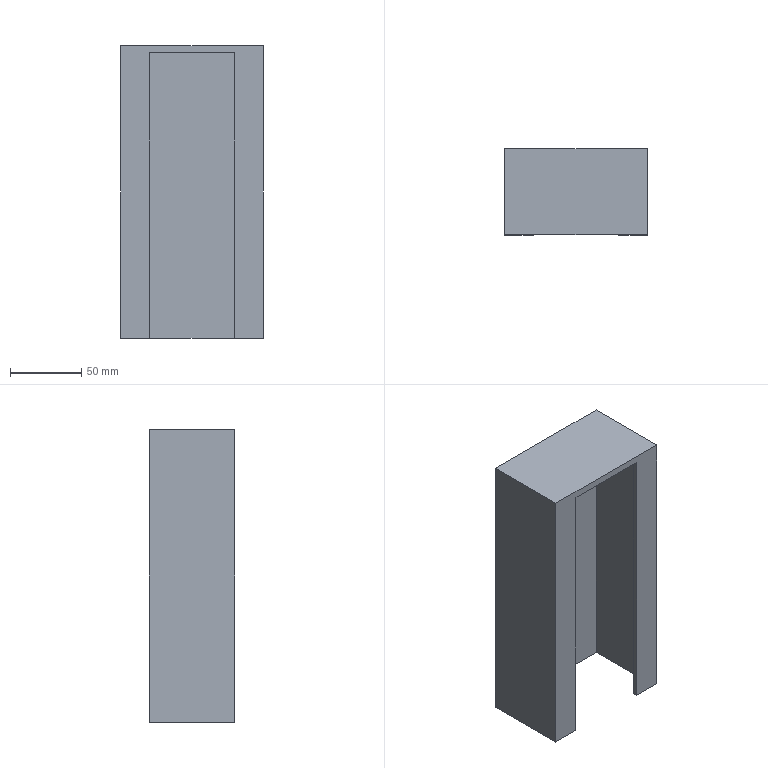Part | STEP file | 1 solid | 14 faces | box 100 x 60 x 205 mm | volume 178800 mm3 | plane 14
STEP:
#1=CARTESIAN_POINT('',(0.,0.,0.));
#2=DIRECTION('',(0.,0.,1.));
#3=DIRECTION('',(1.,0.,0.));
#4=AXIS2_PLACEMENT_3D('',#1,#2,#3);
#5=CARTESIAN_POINT('',(-50.,45.812,205.));
#6=VERTEX_POINT('',#5);
#7=CARTESIAN_POINT('',(50.,45.812,205.));
#8=VERTEX_POINT('',#7);
#9=CARTESIAN_POINT('',(50.,45.812,205.));
#10=DIRECTION('',(1.,0.,0.));
#11=VECTOR('',#10,1.);
#12=LINE('',#9,#11);
#13=CARTESIAN_POINT('',(50.,45.812,0.));
#14=DIRECTION('',(0.,1.,0.));
#15=DIRECTION('',(0.,0.,1.));
#16=AXIS2_PLACEMENT_3D('',#13,#14,#15);
#17=PLANE('',#16);
#18=CARTESIAN_POINT('',(205.,0.));
#19=DIRECTION('',(0.,1.));
#20=VECTOR('',#19,1.);
#21=LINE('',#18,#20);
#22=(GEOMETRIC_REPRESENTATION_CONTEXT(2)PARAMETRIC_REPRESENTATION_CONTEXT()REPRESENTATION_CONTEXT('',''));
#23=DEFINITIONAL_REPRESENTATION('',(#21),#22);
#24=PCURVE('',#17,#23);
#25=CARTESIAN_POINT('',(0.,15.812,205.));
#26=DIRECTION('',(0.,0.,1.));
#27=DIRECTION('',(1.,0.,0.));
#28=AXIS2_PLACEMENT_3D('',#25,#26,#27);
#29=PLANE('',#28);
#30=CARTESIAN_POINT('',(50.,30.));
#31=DIRECTION('',(1.,0.));
#32=VECTOR('',#31,1.);
#33=LINE('',#30,#32);
#34=(GEOMETRIC_REPRESENTATION_CONTEXT(2)PARAMETRIC_REPRESENTATION_CONTEXT()REPRESENTATION_CONTEXT('',''));
#35=DEFINITIONAL_REPRESENTATION('',(#33),#34);
#36=PCURVE('',#29,#35);
#37=SURFACE_CURVE('',#12,(#24,#36),.PCURVE_S1.);
#38=EDGE_CURVE('',#6,#8,#37,.T.);
#39=ORIENTED_EDGE('',*,*,#38,.T.);
#40=CARTESIAN_POINT('',(50.,45.812,0.));
#41=VERTEX_POINT('',#40);
#42=CARTESIAN_POINT('',(50.,45.812,0.));
#43=DIRECTION('',(0.,0.,-1.));
#44=VECTOR('',#43,1.);
#45=LINE('',#42,#44);
#46=CARTESIAN_POINT('',(0.,0.));
#47=DIRECTION('',(-1.,0.));
#48=VECTOR('',#47,1.);
#49=LINE('',#46,#48);
#50=(GEOMETRIC_REPRESENTATION_CONTEXT(2)PARAMETRIC_REPRESENTATION_CONTEXT()REPRESENTATION_CONTEXT('',''));
#51=DEFINITIONAL_REPRESENTATION('',(#49),#50);
#52=PCURVE('',#17,#51);
#53=CARTESIAN_POINT('',(50.,-14.188,0.));
#54=DIRECTION('',(1.,0.,0.));
#55=DIRECTION('',(0.,1.,0.));
#56=AXIS2_PLACEMENT_3D('',#53,#54,#55);
#57=PLANE('',#56);
#58=CARTESIAN_POINT('',(60.,0.));
#59=DIRECTION('',(0.,-1.));
#60=VECTOR('',#59,1.);
#61=LINE('',#58,#60);
#62=(GEOMETRIC_REPRESENTATION_CONTEXT(2)PARAMETRIC_REPRESENTATION_CONTEXT()REPRESENTATION_CONTEXT('',''));
#63=DEFINITIONAL_REPRESENTATION('',(#61),#62);
#64=PCURVE('',#57,#63);
#65=SURFACE_CURVE('',#45,(#52,#64),.PCURVE_S1.);
#66=EDGE_CURVE('',#8,#41,#65,.T.);
#67=ORIENTED_EDGE('',*,*,#66,.T.);
#68=CARTESIAN_POINT('',(-50.,45.812,0.));
#69=VERTEX_POINT('',#68);
#70=CARTESIAN_POINT('',(50.,45.812,0.));
#71=DIRECTION('',(-1.,0.,0.));
#72=VECTOR('',#71,1.);
#73=LINE('',#70,#72);
#74=CARTESIAN_POINT('',(0.,0.));
#75=DIRECTION('',(0.,-1.));
#76=VECTOR('',#75,1.);
#77=LINE('',#74,#76);
#78=(GEOMETRIC_REPRESENTATION_CONTEXT(2)PARAMETRIC_REPRESENTATION_CONTEXT()REPRESENTATION_CONTEXT('',''));
#79=DEFINITIONAL_REPRESENTATION('',(#77),#78);
#80=PCURVE('',#17,#79);
#81=CARTESIAN_POINT('',(0.,22.284,0.));
#82=DIRECTION('',(0.,0.,1.));
#83=DIRECTION('',(1.,0.,0.));
#84=AXIS2_PLACEMENT_3D('',#81,#82,#83);
#85=PLANE('',#84);
#86=CARTESIAN_POINT('',(50.,23.528));
#87=DIRECTION('',(-1.,0.));
#88=VECTOR('',#87,1.);
#89=LINE('',#86,#88);
#90=(GEOMETRIC_REPRESENTATION_CONTEXT(2)PARAMETRIC_REPRESENTATION_CONTEXT()REPRESENTATION_CONTEXT('',''));
#91=DEFINITIONAL_REPRESENTATION('',(#89),#90);
#92=PCURVE('',#85,#91);
#93=SURFACE_CURVE('',#73,(#80,#92),.PCURVE_S1.);
#94=EDGE_CURVE('',#41,#69,#93,.T.);
#95=ORIENTED_EDGE('',*,*,#94,.T.);
#96=CARTESIAN_POINT('',(-50.,45.812,0.));
#97=DIRECTION('',(0.,0.,1.));
#98=VECTOR('',#97,1.);
#99=LINE('',#96,#98);
#100=CARTESIAN_POINT('',(0.,-100.));
#101=DIRECTION('',(1.,0.));
#102=VECTOR('',#101,1.);
#103=LINE('',#100,#102);
#104=(GEOMETRIC_REPRESENTATION_CONTEXT(2)PARAMETRIC_REPRESENTATION_CONTEXT()REPRESENTATION_CONTEXT('',''));
#105=DEFINITIONAL_REPRESENTATION('',(#103),#104);
#106=PCURVE('',#17,#105);
#107=CARTESIAN_POINT('',(-50.,45.812,0.));
#108=DIRECTION('',(-1.,0.,0.));
#109=DIRECTION('',(0.,-1.,0.));
#110=AXIS2_PLACEMENT_3D('',#107,#108,#109);
#111=PLANE('',#110);
#112=CARTESIAN_POINT('',(0.,0.));
#113=DIRECTION('',(0.,1.));
#114=VECTOR('',#113,1.);
#115=LINE('',#112,#114);
#116=(GEOMETRIC_REPRESENTATION_CONTEXT(2)PARAMETRIC_REPRESENTATION_CONTEXT()REPRESENTATION_CONTEXT('',''));
#117=DEFINITIONAL_REPRESENTATION('',(#115),#116);
#118=PCURVE('',#111,#117);
#119=SURFACE_CURVE('',#99,(#106,#118),.PCURVE_S1.);
#120=EDGE_CURVE('',#69,#6,#119,.T.);
#121=ORIENTED_EDGE('',*,*,#120,.T.);
#122=EDGE_LOOP('',(#39,#67,#95,#121));
#123=FACE_BOUND('',#122,.T.);
#124=ADVANCED_FACE('',(#123),#17,.T.);
#125=CARTESIAN_POINT('',(50.,-14.188,205.));
#126=VERTEX_POINT('',#125);
#127=CARTESIAN_POINT('',(50.,-14.188,205.));
#128=DIRECTION('',(0.,-1.,0.));
#129=VECTOR('',#128,1.);
#130=LINE('',#127,#129);
#131=CARTESIAN_POINT('',(0.,205.));
#132=DIRECTION('',(-1.,0.));
#133=VECTOR('',#132,1.);
#134=LINE('',#131,#133);
#135=(GEOMETRIC_REPRESENTATION_CONTEXT(2)PARAMETRIC_REPRESENTATION_CONTEXT()REPRESENTATION_CONTEXT('',''));
#136=DEFINITIONAL_REPRESENTATION('',(#134),#135);
#137=PCURVE('',#57,#136);
#138=CARTESIAN_POINT('',(50.,-30.));
#139=DIRECTION('',(0.,-1.));
#140=VECTOR('',#139,1.);
#141=LINE('',#138,#140);
#142=(GEOMETRIC_REPRESENTATION_CONTEXT(2)PARAMETRIC_REPRESENTATION_CONTEXT()REPRESENTATION_CONTEXT('',''));
#143=DEFINITIONAL_REPRESENTATION('',(#141),#142);
#144=PCURVE('',#29,#143);
#145=SURFACE_CURVE('',#130,(#137,#144),.PCURVE_S1.);
#146=EDGE_CURVE('',#8,#126,#145,.T.);
#147=ORIENTED_EDGE('',*,*,#146,.T.);
#148=CARTESIAN_POINT('',(50.,-14.188,0.));
#149=VERTEX_POINT('',#148);
#150=CARTESIAN_POINT('',(50.,-14.188,0.));
#151=DIRECTION('',(0.,0.,-1.));
#152=VECTOR('',#151,1.);
#153=LINE('',#150,#152);
#154=CARTESIAN_POINT('',(0.,0.));
#155=DIRECTION('',(0.,-1.));
#156=VECTOR('',#155,1.);
#157=LINE('',#154,#156);
#158=(GEOMETRIC_REPRESENTATION_CONTEXT(2)PARAMETRIC_REPRESENTATION_CONTEXT()REPRESENTATION_CONTEXT('',''));
#159=DEFINITIONAL_REPRESENTATION('',(#157),#158);
#160=PCURVE('',#57,#159);
#161=CARTESIAN_POINT('',(30.,-14.188,0.));
#162=DIRECTION('',(0.,-1.,0.));
#163=DIRECTION('',(1.,0.,0.));
#164=AXIS2_PLACEMENT_3D('',#161,#162,#163);
#165=PLANE('',#164);
#166=CARTESIAN_POINT('',(20.,0.));
#167=DIRECTION('',(0.,-1.));
#168=VECTOR('',#167,1.);
#169=LINE('',#166,#168);
#170=(GEOMETRIC_REPRESENTATION_CONTEXT(2)PARAMETRIC_REPRESENTATION_CONTEXT()REPRESENTATION_CONTEXT('',''));
#171=DEFINITIONAL_REPRESENTATION('',(#169),#170);
#172=PCURVE('',#165,#171);
#173=SURFACE_CURVE('',#153,(#160,#172),.PCURVE_S1.);
#174=EDGE_CURVE('',#126,#149,#173,.T.);
#175=ORIENTED_EDGE('',*,*,#174,.T.);
#176=CARTESIAN_POINT('',(50.,-14.188,0.));
#177=DIRECTION('',(0.,1.,0.));
#178=VECTOR('',#177,1.);
#179=LINE('',#176,#178);
#180=CARTESIAN_POINT('',(0.,0.));
#181=DIRECTION('',(1.,0.));
#182=VECTOR('',#181,1.);
#183=LINE('',#180,#182);
#184=(GEOMETRIC_REPRESENTATION_CONTEXT(2)PARAMETRIC_REPRESENTATION_CONTEXT()REPRESENTATION_CONTEXT('',''));
#185=DEFINITIONAL_REPRESENTATION('',(#183),#184);
#186=PCURVE('',#57,#185);
#187=CARTESIAN_POINT('',(50.,-36.472));
#188=DIRECTION('',(0.,1.));
#189=VECTOR('',#188,1.);
#190=LINE('',#187,#189);
#191=(GEOMETRIC_REPRESENTATION_CONTEXT(2)PARAMETRIC_REPRESENTATION_CONTEXT()REPRESENTATION_CONTEXT('',''));
#192=DEFINITIONAL_REPRESENTATION('',(#190),#191);
#193=PCURVE('',#85,#192);
#194=SURFACE_CURVE('',#179,(#186,#193),.PCURVE_S1.);
#195=EDGE_CURVE('',#149,#41,#194,.T.);
#196=ORIENTED_EDGE('',*,*,#195,.T.);
#197=ORIENTED_EDGE('',*,*,#66,.F.);
#198=EDGE_LOOP('',(#147,#175,#196,#197));
#199=FACE_BOUND('',#198,.T.);
#200=ADVANCED_FACE('',(#199),#57,.T.);
#201=ORIENTED_EDGE('',*,*,#146,.F.);
#202=ORIENTED_EDGE('',*,*,#38,.F.);
#203=CARTESIAN_POINT('',(-50.,-14.188,205.));
#204=VERTEX_POINT('',#203);
#205=CARTESIAN_POINT('',(-50.,15.812,205.));
#206=DIRECTION('',(0.,-1.,0.));
#207=VECTOR('',#206,1.);
#208=LINE('',#205,#207);
#209=CARTESIAN_POINT('',(-50.,0.));
#210=DIRECTION('',(0.,-1.));
#211=VECTOR('',#210,1.);
#212=LINE('',#209,#211);
#213=(GEOMETRIC_REPRESENTATION_CONTEXT(2)PARAMETRIC_REPRESENTATION_CONTEXT()REPRESENTATION_CONTEXT('',''));
#214=DEFINITIONAL_REPRESENTATION('',(#212),#213);
#215=PCURVE('',#29,#214);
#216=CARTESIAN_POINT('',(30.,205.));
#217=DIRECTION('',(1.,0.));
#218=VECTOR('',#217,1.);
#219=LINE('',#216,#218);
#220=(GEOMETRIC_REPRESENTATION_CONTEXT(2)PARAMETRIC_REPRESENTATION_CONTEXT()REPRESENTATION_CONTEXT('',''));
#221=DEFINITIONAL_REPRESENTATION('',(#219),#220);
#222=PCURVE('',#111,#221);
#223=SURFACE_CURVE('',#208,(#215,#222),.PCURVE_S1.);
#224=EDGE_CURVE('',#6,#204,#223,.T.);
#225=ORIENTED_EDGE('',*,*,#224,.T.);
#226=CARTESIAN_POINT('',(0.,-14.188,205.));
#227=DIRECTION('',(1.,0.,0.));
#228=VECTOR('',#227,1.);
#229=LINE('',#226,#228);
#230=CARTESIAN_POINT('',(0.,-30.));
#231=DIRECTION('',(1.,0.));
#232=VECTOR('',#231,1.);
#233=LINE('',#230,#232);
#234=(GEOMETRIC_REPRESENTATION_CONTEXT(2)PARAMETRIC_REPRESENTATION_CONTEXT()REPRESENTATION_CONTEXT('',''));
#235=DEFINITIONAL_REPRESENTATION('',(#233),#234);
#236=PCURVE('',#29,#235);
#237=CARTESIAN_POINT('',(-30.,205.));
#238=DIRECTION('',(1.,0.));
#239=VECTOR('',#238,1.);
#240=LINE('',#237,#239);
#241=(GEOMETRIC_REPRESENTATION_CONTEXT(2)PARAMETRIC_REPRESENTATION_CONTEXT()REPRESENTATION_CONTEXT('',''));
#242=DEFINITIONAL_REPRESENTATION('',(#240),#241);
#243=PCURVE('',#165,#242);
#244=SURFACE_CURVE('',#229,(#236,#243),.PCURVE_S1.);
#245=EDGE_CURVE('',#204,#126,#244,.T.);
#246=ORIENTED_EDGE('',*,*,#245,.T.);
#247=EDGE_LOOP('',(#201,#202,#225,#246));
#248=FACE_BOUND('',#247,.T.);
#249=ADVANCED_FACE('',(#248),#29,.T.);
#250=ORIENTED_EDGE('',*,*,#224,.F.);
#251=ORIENTED_EDGE('',*,*,#120,.F.);
#252=CARTESIAN_POINT('',(-50.,-14.188,0.));
#253=VERTEX_POINT('',#252);
#254=CARTESIAN_POINT('',(-50.,45.812,0.));
#255=DIRECTION('',(0.,-1.,0.));
#256=VECTOR('',#255,1.);
#257=LINE('',#254,#256);
#258=CARTESIAN_POINT('',(0.,0.));
#259=DIRECTION('',(1.,0.));
#260=VECTOR('',#259,1.);
#261=LINE('',#258,#260);
#262=(GEOMETRIC_REPRESENTATION_CONTEXT(2)PARAMETRIC_REPRESENTATION_CONTEXT()REPRESENTATION_CONTEXT('',''));
#263=DEFINITIONAL_REPRESENTATION('',(#261),#262);
#264=PCURVE('',#111,#263);
#265=CARTESIAN_POINT('',(-50.,23.528));
#266=DIRECTION('',(0.,-1.));
#267=VECTOR('',#266,1.);
#268=LINE('',#265,#267);
#269=(GEOMETRIC_REPRESENTATION_CONTEXT(2)PARAMETRIC_REPRESENTATION_CONTEXT()REPRESENTATION_CONTEXT('',''));
#270=DEFINITIONAL_REPRESENTATION('',(#268),#269);
#271=PCURVE('',#85,#270);
#272=SURFACE_CURVE('',#257,(#264,#271),.PCURVE_S1.);
#273=EDGE_CURVE('',#69,#253,#272,.T.);
#274=ORIENTED_EDGE('',*,*,#273,.T.);
#275=CARTESIAN_POINT('',(-50.,-14.188,0.));
#276=DIRECTION('',(0.,0.,1.));
#277=VECTOR('',#276,1.);
#278=LINE('',#275,#277);
#279=CARTESIAN_POINT('',(60.,0.));
#280=DIRECTION('',(0.,1.));
#281=VECTOR('',#280,1.);
#282=LINE('',#279,#281);
#283=(GEOMETRIC_REPRESENTATION_CONTEXT(2)PARAMETRIC_REPRESENTATION_CONTEXT()REPRESENTATION_CONTEXT('',''));
#284=DEFINITIONAL_REPRESENTATION('',(#282),#283);
#285=PCURVE('',#111,#284);
#286=CARTESIAN_POINT('',(-80.,0.));
#287=DIRECTION('',(0.,1.));
#288=VECTOR('',#287,1.);
#289=LINE('',#286,#288);
#290=(GEOMETRIC_REPRESENTATION_CONTEXT(2)PARAMETRIC_REPRESENTATION_CONTEXT()REPRESENTATION_CONTEXT('',''));
#291=DEFINITIONAL_REPRESENTATION('',(#289),#290);
#292=PCURVE('',#165,#291);
#293=SURFACE_CURVE('',#278,(#285,#292),.PCURVE_S1.);
#294=EDGE_CURVE('',#253,#204,#293,.T.);
#295=ORIENTED_EDGE('',*,*,#294,.T.);
#296=EDGE_LOOP('',(#250,#251,#274,#295));
#297=FACE_BOUND('',#296,.T.);
#298=ADVANCED_FACE('',(#297),#111,.T.);
#299=ORIENTED_EDGE('',*,*,#195,.F.);
#300=CARTESIAN_POINT('',(30.,-14.188,0.));
#301=VERTEX_POINT('',#300);
#302=CARTESIAN_POINT('',(0.,-14.188,0.));
#303=DIRECTION('',(1.,0.,0.));
#304=VECTOR('',#303,1.);
#305=LINE('',#302,#304);
#306=CARTESIAN_POINT('',(0.,-36.472));
#307=DIRECTION('',(1.,0.));
#308=VECTOR('',#307,1.);
#309=LINE('',#306,#308);
#310=(GEOMETRIC_REPRESENTATION_CONTEXT(2)PARAMETRIC_REPRESENTATION_CONTEXT()REPRESENTATION_CONTEXT('',''));
#311=DEFINITIONAL_REPRESENTATION('',(#309),#310);
#312=PCURVE('',#85,#311);
#313=CARTESIAN_POINT('',(-30.,0.));
#314=DIRECTION('',(1.,0.));
#315=VECTOR('',#314,1.);
#316=LINE('',#313,#315);
#317=(GEOMETRIC_REPRESENTATION_CONTEXT(2)PARAMETRIC_REPRESENTATION_CONTEXT()REPRESENTATION_CONTEXT('',''));
#318=DEFINITIONAL_REPRESENTATION('',(#316),#317);
#319=PCURVE('',#165,#318);
#320=SURFACE_CURVE('',#305,(#312,#319),.PCURVE_S1.);
#321=EDGE_CURVE('',#301,#149,#320,.T.);
#322=ORIENTED_EDGE('',*,*,#321,.F.);
#323=CARTESIAN_POINT('',(30.,-11.188,0.));
#324=VERTEX_POINT('',#323);
#325=CARTESIAN_POINT('',(30.,22.284,0.));
#326=DIRECTION('',(0.,-1.,0.));
#327=VECTOR('',#326,1.);
#328=LINE('',#325,#327);
#329=CARTESIAN_POINT('',(30.,0.));
#330=DIRECTION('',(0.,-1.));
#331=VECTOR('',#330,1.);
#332=LINE('',#329,#331);
#333=(GEOMETRIC_REPRESENTATION_CONTEXT(2)PARAMETRIC_REPRESENTATION_CONTEXT()REPRESENTATION_CONTEXT('',''));
#334=DEFINITIONAL_REPRESENTATION('',(#332),#333);
#335=PCURVE('',#85,#334);
#336=CARTESIAN_POINT('',(30.,-11.188,0.));
#337=DIRECTION('',(-1.,0.,0.));
#338=DIRECTION('',(0.,0.,1.));
#339=AXIS2_PLACEMENT_3D('',#336,#337,#338);
#340=PLANE('',#339);
#341=CARTESIAN_POINT('',(0.,33.472));
#342=DIRECTION('',(0.,-1.));
#343=VECTOR('',#342,1.);
#344=LINE('',#341,#343);
#345=(GEOMETRIC_REPRESENTATION_CONTEXT(2)PARAMETRIC_REPRESENTATION_CONTEXT()REPRESENTATION_CONTEXT('',''));
#346=DEFINITIONAL_REPRESENTATION('',(#344),#345);
#347=PCURVE('',#340,#346);
#348=SURFACE_CURVE('',#328,(#335,#347),.PCURVE_S1.);
#349=EDGE_CURVE('',#324,#301,#348,.T.);
#350=ORIENTED_EDGE('',*,*,#349,.F.);
#351=CARTESIAN_POINT('',(47.,-11.188,0.));
#352=VERTEX_POINT('',#351);
#353=CARTESIAN_POINT('',(0.,-11.188,0.));
#354=DIRECTION('',(-1.,0.,0.));
#355=VECTOR('',#354,1.);
#356=LINE('',#353,#355);
#357=CARTESIAN_POINT('',(0.,-33.472));
#358=DIRECTION('',(-1.,0.));
#359=VECTOR('',#358,1.);
#360=LINE('',#357,#359);
#361=(GEOMETRIC_REPRESENTATION_CONTEXT(2)PARAMETRIC_REPRESENTATION_CONTEXT()REPRESENTATION_CONTEXT('',''));
#362=DEFINITIONAL_REPRESENTATION('',(#360),#361);
#363=PCURVE('',#85,#362);
#364=CARTESIAN_POINT('',(47.,-11.188,0.));
#365=DIRECTION('',(0.,1.,0.));
#366=DIRECTION('',(-1.,0.,0.));
#367=AXIS2_PLACEMENT_3D('',#364,#365,#366);
#368=PLANE('',#367);
#369=CARTESIAN_POINT('',(47.,0.));
#370=DIRECTION('',(1.,0.));
#371=VECTOR('',#370,1.);
#372=LINE('',#369,#371);
#373=(GEOMETRIC_REPRESENTATION_CONTEXT(2)PARAMETRIC_REPRESENTATION_CONTEXT()REPRESENTATION_CONTEXT('',''));
#374=DEFINITIONAL_REPRESENTATION('',(#372),#373);
#375=PCURVE('',#368,#374);
#376=SURFACE_CURVE('',#356,(#363,#375),.PCURVE_S1.);
#377=EDGE_CURVE('',#352,#324,#376,.T.);
#378=ORIENTED_EDGE('',*,*,#377,.F.);
#379=CARTESIAN_POINT('',(47.,42.812,0.));
#380=VERTEX_POINT('',#379);
#381=CARTESIAN_POINT('',(47.,22.284,0.));
#382=DIRECTION('',(0.,-1.,0.));
#383=VECTOR('',#382,1.);
#384=LINE('',#381,#383);
#385=CARTESIAN_POINT('',(47.,0.));
#386=DIRECTION('',(0.,-1.));
#387=VECTOR('',#386,1.);
#388=LINE('',#385,#387);
#389=(GEOMETRIC_REPRESENTATION_CONTEXT(2)PARAMETRIC_REPRESENTATION_CONTEXT()REPRESENTATION_CONTEXT('',''));
#390=DEFINITIONAL_REPRESENTATION('',(#388),#389);
#391=PCURVE('',#85,#390);
#392=CARTESIAN_POINT('',(47.,42.812,0.));
#393=DIRECTION('',(-1.,0.,0.));
#394=DIRECTION('',(0.,-1.,0.));
#395=AXIS2_PLACEMENT_3D('',#392,#393,#394);
#396=PLANE('',#395);
#397=CARTESIAN_POINT('',(20.528,0.));
#398=DIRECTION('',(1.,0.));
#399=VECTOR('',#398,1.);
#400=LINE('',#397,#399);
#401=(GEOMETRIC_REPRESENTATION_CONTEXT(2)PARAMETRIC_REPRESENTATION_CONTEXT()REPRESENTATION_CONTEXT('',''));
#402=DEFINITIONAL_REPRESENTATION('',(#400),#401);
#403=PCURVE('',#396,#402);
#404=SURFACE_CURVE('',#384,(#391,#403),.PCURVE_S1.);
#405=EDGE_CURVE('',#380,#352,#404,.T.);
#406=ORIENTED_EDGE('',*,*,#405,.F.);
#407=CARTESIAN_POINT('',(-47.,42.812,0.));
#408=VERTEX_POINT('',#407);
#409=CARTESIAN_POINT('',(0.,42.812,0.));
#410=DIRECTION('',(1.,0.,0.));
#411=VECTOR('',#410,1.);
#412=LINE('',#409,#411);
#413=CARTESIAN_POINT('',(0.,20.528));
#414=DIRECTION('',(1.,0.));
#415=VECTOR('',#414,1.);
#416=LINE('',#413,#415);
#417=(GEOMETRIC_REPRESENTATION_CONTEXT(2)PARAMETRIC_REPRESENTATION_CONTEXT()REPRESENTATION_CONTEXT('',''));
#418=DEFINITIONAL_REPRESENTATION('',(#416),#417);
#419=PCURVE('',#85,#418);
#420=CARTESIAN_POINT('',(-47.,42.812,0.));
#421=DIRECTION('',(0.,-1.,0.));
#422=DIRECTION('',(0.,0.,-1.));
#423=AXIS2_PLACEMENT_3D('',#420,#421,#422);
#424=PLANE('',#423);
#425=CARTESIAN_POINT('',(0.,47.));
#426=DIRECTION('',(0.,1.));
#427=VECTOR('',#426,1.);
#428=LINE('',#425,#427);
#429=(GEOMETRIC_REPRESENTATION_CONTEXT(2)PARAMETRIC_REPRESENTATION_CONTEXT()REPRESENTATION_CONTEXT('',''));
#430=DEFINITIONAL_REPRESENTATION('',(#428),#429);
#431=PCURVE('',#424,#430);
#432=SURFACE_CURVE('',#412,(#419,#431),.PCURVE_S1.);
#433=EDGE_CURVE('',#408,#380,#432,.T.);
#434=ORIENTED_EDGE('',*,*,#433,.F.);
#435=CARTESIAN_POINT('',(-47.,-11.188,0.));
#436=VERTEX_POINT('',#435);
#437=CARTESIAN_POINT('',(-47.,22.284,0.));
#438=DIRECTION('',(0.,1.,0.));
#439=VECTOR('',#438,1.);
#440=LINE('',#437,#439);
#441=CARTESIAN_POINT('',(-47.,0.));
#442=DIRECTION('',(0.,1.));
#443=VECTOR('',#442,1.);
#444=LINE('',#441,#443);
#445=(GEOMETRIC_REPRESENTATION_CONTEXT(2)PARAMETRIC_REPRESENTATION_CONTEXT()REPRESENTATION_CONTEXT('',''));
#446=DEFINITIONAL_REPRESENTATION('',(#444),#445);
#447=PCURVE('',#85,#446);
#448=CARTESIAN_POINT('',(-47.,-11.188,0.));
#449=DIRECTION('',(1.,0.,0.));
#450=DIRECTION('',(0.,1.,0.));
#451=AXIS2_PLACEMENT_3D('',#448,#449,#450);
#452=PLANE('',#451);
#453=CARTESIAN_POINT('',(33.472,0.));
#454=DIRECTION('',(1.,0.));
#455=VECTOR('',#454,1.);
#456=LINE('',#453,#455);
#457=(GEOMETRIC_REPRESENTATION_CONTEXT(2)PARAMETRIC_REPRESENTATION_CONTEXT()REPRESENTATION_CONTEXT('',''));
#458=DEFINITIONAL_REPRESENTATION('',(#456),#457);
#459=PCURVE('',#452,#458);
#460=SURFACE_CURVE('',#440,(#447,#459),.PCURVE_S1.);
#461=EDGE_CURVE('',#436,#408,#460,.T.);
#462=ORIENTED_EDGE('',*,*,#461,.F.);
#463=CARTESIAN_POINT('',(-30.,-11.188,0.));
#464=VERTEX_POINT('',#463);
#465=CARTESIAN_POINT('',(0.,-11.188,0.));
#466=DIRECTION('',(-1.,0.,0.));
#467=VECTOR('',#466,1.);
#468=LINE('',#465,#467);
#469=CARTESIAN_POINT('',(0.,-33.472));
#470=DIRECTION('',(-1.,0.));
#471=VECTOR('',#470,1.);
#472=LINE('',#469,#471);
#473=(GEOMETRIC_REPRESENTATION_CONTEXT(2)PARAMETRIC_REPRESENTATION_CONTEXT()REPRESENTATION_CONTEXT('',''));
#474=DEFINITIONAL_REPRESENTATION('',(#472),#473);
#475=PCURVE('',#85,#474);
#476=CARTESIAN_POINT('',(-30.,-11.188,0.));
#477=DIRECTION('',(0.,1.,0.));
#478=DIRECTION('',(-1.,0.,0.));
#479=AXIS2_PLACEMENT_3D('',#476,#477,#478);
#480=PLANE('',#479);
#481=CARTESIAN_POINT('',(-30.,0.));
#482=DIRECTION('',(1.,0.));
#483=VECTOR('',#482,1.);
#484=LINE('',#481,#483);
#485=(GEOMETRIC_REPRESENTATION_CONTEXT(2)PARAMETRIC_REPRESENTATION_CONTEXT()REPRESENTATION_CONTEXT('',''));
#486=DEFINITIONAL_REPRESENTATION('',(#484),#485);
#487=PCURVE('',#480,#486);
#488=SURFACE_CURVE('',#468,(#475,#487),.PCURVE_S1.);
#489=EDGE_CURVE('',#464,#436,#488,.T.);
#490=ORIENTED_EDGE('',*,*,#489,.F.);
#491=CARTESIAN_POINT('',(-30.,-14.188,0.));
#492=VERTEX_POINT('',#491);
#493=CARTESIAN_POINT('',(-30.,22.284,0.));
#494=DIRECTION('',(0.,1.,0.));
#495=VECTOR('',#494,1.);
#496=LINE('',#493,#495);
#497=CARTESIAN_POINT('',(-30.,0.));
#498=DIRECTION('',(0.,1.));
#499=VECTOR('',#498,1.);
#500=LINE('',#497,#499);
#501=(GEOMETRIC_REPRESENTATION_CONTEXT(2)PARAMETRIC_REPRESENTATION_CONTEXT()REPRESENTATION_CONTEXT('',''));
#502=DEFINITIONAL_REPRESENTATION('',(#500),#501);
#503=PCURVE('',#85,#502);
#504=CARTESIAN_POINT('',(-30.,-14.188,0.));
#505=DIRECTION('',(1.,0.,0.));
#506=DIRECTION('',(0.,0.,-1.));
#507=AXIS2_PLACEMENT_3D('',#504,#505,#506);
#508=PLANE('',#507);
#509=CARTESIAN_POINT('',(0.,36.472));
#510=DIRECTION('',(0.,1.));
#511=VECTOR('',#510,1.);
#512=LINE('',#509,#511);
#513=(GEOMETRIC_REPRESENTATION_CONTEXT(2)PARAMETRIC_REPRESENTATION_CONTEXT()REPRESENTATION_CONTEXT('',''));
#514=DEFINITIONAL_REPRESENTATION('',(#512),#513);
#515=PCURVE('',#508,#514);
#516=SURFACE_CURVE('',#496,(#503,#515),.PCURVE_S1.);
#517=EDGE_CURVE('',#492,#464,#516,.T.);
#518=ORIENTED_EDGE('',*,*,#517,.F.);
#519=CARTESIAN_POINT('',(0.,-14.188,0.));
#520=DIRECTION('',(1.,0.,0.));
#521=VECTOR('',#520,1.);
#522=LINE('',#519,#521);
#523=CARTESIAN_POINT('',(0.,-36.472));
#524=DIRECTION('',(1.,0.));
#525=VECTOR('',#524,1.);
#526=LINE('',#523,#525);
#527=(GEOMETRIC_REPRESENTATION_CONTEXT(2)PARAMETRIC_REPRESENTATION_CONTEXT()REPRESENTATION_CONTEXT('',''));
#528=DEFINITIONAL_REPRESENTATION('',(#526),#527);
#529=PCURVE('',#85,#528);
#530=CARTESIAN_POINT('',(-30.,0.));
#531=DIRECTION('',(1.,0.));
#532=VECTOR('',#531,1.);
#533=LINE('',#530,#532);
#534=(GEOMETRIC_REPRESENTATION_CONTEXT(2)PARAMETRIC_REPRESENTATION_CONTEXT()REPRESENTATION_CONTEXT('',''));
#535=DEFINITIONAL_REPRESENTATION('',(#533),#534);
#536=PCURVE('',#165,#535);
#537=SURFACE_CURVE('',#522,(#529,#536),.PCURVE_S1.);
#538=EDGE_CURVE('',#253,#492,#537,.T.);
#539=ORIENTED_EDGE('',*,*,#538,.F.);
#540=ORIENTED_EDGE('',*,*,#273,.F.);
#541=ORIENTED_EDGE('',*,*,#94,.F.);
#542=EDGE_LOOP('',(#299,#322,#350,#378,#406,#434,#462,#490,#518,#539,#540,#541));
#543=FACE_BOUND('',#542,.T.);
#544=ADVANCED_FACE('',(#543),#85,.F.);
#545=CARTESIAN_POINT('',(-30.,-14.188,200.));
#546=VERTEX_POINT('',#545);
#547=CARTESIAN_POINT('',(30.,-14.188,200.));
#548=VERTEX_POINT('',#547);
#549=CARTESIAN_POINT('',(30.,-14.188,200.));
#550=DIRECTION('',(1.,0.,0.));
#551=VECTOR('',#550,1.);
#552=LINE('',#549,#551);
#553=CARTESIAN_POINT('',(0.,200.));
#554=DIRECTION('',(1.,0.));
#555=VECTOR('',#554,1.);
#556=LINE('',#553,#555);
#557=(GEOMETRIC_REPRESENTATION_CONTEXT(2)PARAMETRIC_REPRESENTATION_CONTEXT()REPRESENTATION_CONTEXT('',''));
#558=DEFINITIONAL_REPRESENTATION('',(#556),#557);
#559=PCURVE('',#165,#558);
#560=CARTESIAN_POINT('',(0.,15.812,200.));
#561=DIRECTION('',(0.,0.,1.));
#562=DIRECTION('',(1.,0.,0.));
#563=AXIS2_PLACEMENT_3D('',#560,#561,#562);
#564=PLANE('',#563);
#565=CARTESIAN_POINT('',(30.,-30.));
#566=DIRECTION('',(1.,0.));
#567=VECTOR('',#566,1.);
#568=LINE('',#565,#567);
#569=(GEOMETRIC_REPRESENTATION_CONTEXT(2)PARAMETRIC_REPRESENTATION_CONTEXT()REPRESENTATION_CONTEXT('',''));
#570=DEFINITIONAL_REPRESENTATION('',(#568),#569);
#571=PCURVE('',#564,#570);
#572=SURFACE_CURVE('',#552,(#559,#571),.PCURVE_S1.);
#573=EDGE_CURVE('',#546,#548,#572,.T.);
#574=ORIENTED_EDGE('',*,*,#573,.T.);
#575=CARTESIAN_POINT('',(30.,-14.188,0.));
#576=DIRECTION('',(0.,0.,-1.));
#577=VECTOR('',#576,1.);
#578=LINE('',#575,#577);
#579=CARTESIAN_POINT('',(0.,0.));
#580=DIRECTION('',(0.,-1.));
#581=VECTOR('',#580,1.);
#582=LINE('',#579,#581);
#583=(GEOMETRIC_REPRESENTATION_CONTEXT(2)PARAMETRIC_REPRESENTATION_CONTEXT()REPRESENTATION_CONTEXT('',''));
#584=DEFINITIONAL_REPRESENTATION('',(#582),#583);
#585=PCURVE('',#165,#584);
#586=CARTESIAN_POINT('',(0.,-3.));
#587=DIRECTION('',(-1.,0.));
#588=VECTOR('',#587,1.);
#589=LINE('',#586,#588);
#590=(GEOMETRIC_REPRESENTATION_CONTEXT(2)PARAMETRIC_REPRESENTATION_CONTEXT()REPRESENTATION_CONTEXT('',''));
#591=DEFINITIONAL_REPRESENTATION('',(#589),#590);
#592=PCURVE('',#340,#591);
#593=SURFACE_CURVE('',#578,(#585,#592),.PCURVE_S1.);
#594=EDGE_CURVE('',#548,#301,#593,.T.);
#595=ORIENTED_EDGE('',*,*,#594,.T.);
#596=ORIENTED_EDGE('',*,*,#321,.T.);
#597=ORIENTED_EDGE('',*,*,#174,.F.);
#598=ORIENTED_EDGE('',*,*,#245,.F.);
#599=ORIENTED_EDGE('',*,*,#294,.F.);
#600=ORIENTED_EDGE('',*,*,#538,.T.);
#601=CARTESIAN_POINT('',(-30.,-14.188,0.));
#602=DIRECTION('',(0.,0.,1.));
#603=VECTOR('',#602,1.);
#604=LINE('',#601,#603);
#605=CARTESIAN_POINT('',(-60.,0.));
#606=DIRECTION('',(0.,1.));
#607=VECTOR('',#606,1.);
#608=LINE('',#605,#607);
#609=(GEOMETRIC_REPRESENTATION_CONTEXT(2)PARAMETRIC_REPRESENTATION_CONTEXT()REPRESENTATION_CONTEXT('',''));
#610=DEFINITIONAL_REPRESENTATION('',(#608),#609);
#611=PCURVE('',#165,#610);
#612=CARTESIAN_POINT('',(0.,0.));
#613=DIRECTION('',(-1.,0.));
#614=VECTOR('',#613,1.);
#615=LINE('',#612,#614);
#616=(GEOMETRIC_REPRESENTATION_CONTEXT(2)PARAMETRIC_REPRESENTATION_CONTEXT()REPRESENTATION_CONTEXT('',''));
#617=DEFINITIONAL_REPRESENTATION('',(#615),#616);
#618=PCURVE('',#508,#617);
#619=SURFACE_CURVE('',#604,(#611,#618),.PCURVE_S1.);
#620=EDGE_CURVE('',#492,#546,#619,.T.);
#621=ORIENTED_EDGE('',*,*,#620,.T.);
#622=EDGE_LOOP('',(#574,#595,#596,#597,#598,#599,#600,#621));
#623=FACE_BOUND('',#622,.T.);
#624=ADVANCED_FACE('',(#623),#165,.T.);
#625=CARTESIAN_POINT('',(30.,-11.188,200.));
#626=VERTEX_POINT('',#625);
#627=CARTESIAN_POINT('',(30.,-11.188,200.));
#628=DIRECTION('',(0.,1.,0.));
#629=VECTOR('',#628,1.);
#630=LINE('',#627,#629);
#631=CARTESIAN_POINT('',(200.,0.));
#632=DIRECTION('',(0.,1.));
#633=VECTOR('',#632,1.);
#634=LINE('',#631,#633);
#635=(GEOMETRIC_REPRESENTATION_CONTEXT(2)PARAMETRIC_REPRESENTATION_CONTEXT()REPRESENTATION_CONTEXT('',''));
#636=DEFINITIONAL_REPRESENTATION('',(#634),#635);
#637=PCURVE('',#340,#636);
#638=CARTESIAN_POINT('',(30.,-27.));
#639=DIRECTION('',(0.,1.));
#640=VECTOR('',#639,1.);
#641=LINE('',#638,#640);
#642=(GEOMETRIC_REPRESENTATION_CONTEXT(2)PARAMETRIC_REPRESENTATION_CONTEXT()REPRESENTATION_CONTEXT('',''));
#643=DEFINITIONAL_REPRESENTATION('',(#641),#642);
#644=PCURVE('',#564,#643);
#645=SURFACE_CURVE('',#630,(#637,#644),.PCURVE_S1.);
#646=EDGE_CURVE('',#548,#626,#645,.T.);
#647=ORIENTED_EDGE('',*,*,#646,.T.);
#648=CARTESIAN_POINT('',(30.,-11.188,0.));
#649=DIRECTION('',(0.,0.,-1.));
#650=VECTOR('',#649,1.);
#651=LINE('',#648,#650);
#652=CARTESIAN_POINT('',(0.,0.));
#653=DIRECTION('',(-1.,0.));
#654=VECTOR('',#653,1.);
#655=LINE('',#652,#654);
#656=(GEOMETRIC_REPRESENTATION_CONTEXT(2)PARAMETRIC_REPRESENTATION_CONTEXT()REPRESENTATION_CONTEXT('',''));
#657=DEFINITIONAL_REPRESENTATION('',(#655),#656);
#658=PCURVE('',#340,#657);
#659=CARTESIAN_POINT('',(17.,0.));
#660=DIRECTION('',(0.,-1.));
#661=VECTOR('',#660,1.);
#662=LINE('',#659,#661);
#663=(GEOMETRIC_REPRESENTATION_CONTEXT(2)PARAMETRIC_REPRESENTATION_CONTEXT()REPRESENTATION_CONTEXT('',''));
#664=DEFINITIONAL_REPRESENTATION('',(#662),#663);
#665=PCURVE('',#368,#664);
#666=SURFACE_CURVE('',#651,(#658,#665),.PCURVE_S1.);
#667=EDGE_CURVE('',#626,#324,#666,.T.);
#668=ORIENTED_EDGE('',*,*,#667,.T.);
#669=ORIENTED_EDGE('',*,*,#349,.T.);
#670=ORIENTED_EDGE('',*,*,#594,.F.);
#671=EDGE_LOOP('',(#647,#668,#669,#670));
#672=FACE_BOUND('',#671,.T.);
#673=ADVANCED_FACE('',(#672),#340,.T.);
#674=CARTESIAN_POINT('',(47.,-11.188,200.));
#675=VERTEX_POINT('',#674);
#676=CARTESIAN_POINT('',(47.,-11.188,200.));
#677=DIRECTION('',(1.,0.,0.));
#678=VECTOR('',#677,1.);
#679=LINE('',#676,#678);
#680=CARTESIAN_POINT('',(0.,200.));
#681=DIRECTION('',(-1.,0.));
#682=VECTOR('',#681,1.);
#683=LINE('',#680,#682);
#684=(GEOMETRIC_REPRESENTATION_CONTEXT(2)PARAMETRIC_REPRESENTATION_CONTEXT()REPRESENTATION_CONTEXT('',''));
#685=DEFINITIONAL_REPRESENTATION('',(#683),#684);
#686=PCURVE('',#368,#685);
#687=CARTESIAN_POINT('',(47.,-27.));
#688=DIRECTION('',(1.,0.));
#689=VECTOR('',#688,1.);
#690=LINE('',#687,#689);
#691=(GEOMETRIC_REPRESENTATION_CONTEXT(2)PARAMETRIC_REPRESENTATION_CONTEXT()REPRESENTATION_CONTEXT('',''));
#692=DEFINITIONAL_REPRESENTATION('',(#690),#691);
#693=PCURVE('',#564,#692);
#694=SURFACE_CURVE('',#679,(#686,#693),.PCURVE_S1.);
#695=EDGE_CURVE('',#626,#675,#694,.T.);
#696=ORIENTED_EDGE('',*,*,#695,.T.);
#697=CARTESIAN_POINT('',(47.,-11.188,0.));
#698=DIRECTION('',(0.,0.,-1.));
#699=VECTOR('',#698,1.);
#700=LINE('',#697,#699);
#701=CARTESIAN_POINT('',(0.,0.));
#702=DIRECTION('',(0.,-1.));
#703=VECTOR('',#702,1.);
#704=LINE('',#701,#703);
#705=(GEOMETRIC_REPRESENTATION_CONTEXT(2)PARAMETRIC_REPRESENTATION_CONTEXT()REPRESENTATION_CONTEXT('',''));
#706=DEFINITIONAL_REPRESENTATION('',(#704),#705);
#707=PCURVE('',#368,#706);
#708=CARTESIAN_POINT('',(54.,0.));
#709=DIRECTION('',(0.,-1.));
#710=VECTOR('',#709,1.);
#711=LINE('',#708,#710);
#712=(GEOMETRIC_REPRESENTATION_CONTEXT(2)PARAMETRIC_REPRESENTATION_CONTEXT()REPRESENTATION_CONTEXT('',''));
#713=DEFINITIONAL_REPRESENTATION('',(#711),#712);
#714=PCURVE('',#396,#713);
#715=SURFACE_CURVE('',#700,(#707,#714),.PCURVE_S1.);
#716=EDGE_CURVE('',#675,#352,#715,.T.);
#717=ORIENTED_EDGE('',*,*,#716,.T.);
#718=ORIENTED_EDGE('',*,*,#377,.T.);
#719=ORIENTED_EDGE('',*,*,#667,.F.);
#720=EDGE_LOOP('',(#696,#717,#718,#719));
#721=FACE_BOUND('',#720,.T.);
#722=ADVANCED_FACE('',(#721),#368,.T.);
#723=CARTESIAN_POINT('',(47.,42.812,200.));
#724=VERTEX_POINT('',#723);
#725=CARTESIAN_POINT('',(47.,42.812,200.));
#726=DIRECTION('',(0.,1.,0.));
#727=VECTOR('',#726,1.);
#728=LINE('',#725,#727);
#729=CARTESIAN_POINT('',(0.,200.));
#730=DIRECTION('',(-1.,0.));
#731=VECTOR('',#730,1.);
#732=LINE('',#729,#731);
#733=(GEOMETRIC_REPRESENTATION_CONTEXT(2)PARAMETRIC_REPRESENTATION_CONTEXT()REPRESENTATION_CONTEXT('',''));
#734=DEFINITIONAL_REPRESENTATION('',(#732),#733);
#735=PCURVE('',#396,#734);
#736=CARTESIAN_POINT('',(47.,27.));
#737=DIRECTION('',(0.,1.));
#738=VECTOR('',#737,1.);
#739=LINE('',#736,#738);
#740=(GEOMETRIC_REPRESENTATION_CONTEXT(2)PARAMETRIC_REPRESENTATION_CONTEXT()REPRESENTATION_CONTEXT('',''));
#741=DEFINITIONAL_REPRESENTATION('',(#739),#740);
#742=PCURVE('',#564,#741);
#743=SURFACE_CURVE('',#728,(#735,#742),.PCURVE_S1.);
#744=EDGE_CURVE('',#675,#724,#743,.T.);
#745=ORIENTED_EDGE('',*,*,#744,.T.);
#746=CARTESIAN_POINT('',(47.,42.812,0.));
#747=DIRECTION('',(0.,0.,-1.));
#748=VECTOR('',#747,1.);
#749=LINE('',#746,#748);
#750=CARTESIAN_POINT('',(0.,0.));
#751=DIRECTION('',(0.,-1.));
#752=VECTOR('',#751,1.);
#753=LINE('',#750,#752);
#754=(GEOMETRIC_REPRESENTATION_CONTEXT(2)PARAMETRIC_REPRESENTATION_CONTEXT()REPRESENTATION_CONTEXT('',''));
#755=DEFINITIONAL_REPRESENTATION('',(#753),#754);
#756=PCURVE('',#396,#755);
#757=CARTESIAN_POINT('',(0.,94.));
#758=DIRECTION('',(1.,0.));
#759=VECTOR('',#758,1.);
#760=LINE('',#757,#759);
#761=(GEOMETRIC_REPRESENTATION_CONTEXT(2)PARAMETRIC_REPRESENTATION_CONTEXT()REPRESENTATION_CONTEXT('',''));
#762=DEFINITIONAL_REPRESENTATION('',(#760),#761);
#763=PCURVE('',#424,#762);
#764=SURFACE_CURVE('',#749,(#756,#763),.PCURVE_S1.);
#765=EDGE_CURVE('',#724,#380,#764,.T.);
#766=ORIENTED_EDGE('',*,*,#765,.T.);
#767=ORIENTED_EDGE('',*,*,#405,.T.);
#768=ORIENTED_EDGE('',*,*,#716,.F.);
#769=EDGE_LOOP('',(#745,#766,#767,#768));
#770=FACE_BOUND('',#769,.T.);
#771=ADVANCED_FACE('',(#770),#396,.T.);
#772=CARTESIAN_POINT('',(-47.,42.812,200.));
#773=VERTEX_POINT('',#772);
#774=CARTESIAN_POINT('',(-47.,42.812,200.));
#775=DIRECTION('',(-1.,0.,0.));
#776=VECTOR('',#775,1.);
#777=LINE('',#774,#776);
#778=CARTESIAN_POINT('',(-200.,0.));
#779=DIRECTION('',(0.,-1.));
#780=VECTOR('',#779,1.);
#781=LINE('',#778,#780);
#782=(GEOMETRIC_REPRESENTATION_CONTEXT(2)PARAMETRIC_REPRESENTATION_CONTEXT()REPRESENTATION_CONTEXT('',''));
#783=DEFINITIONAL_REPRESENTATION('',(#781),#782);
#784=PCURVE('',#424,#783);
#785=CARTESIAN_POINT('',(-47.,27.));
#786=DIRECTION('',(-1.,0.));
#787=VECTOR('',#786,1.);
#788=LINE('',#785,#787);
#789=(GEOMETRIC_REPRESENTATION_CONTEXT(2)PARAMETRIC_REPRESENTATION_CONTEXT()REPRESENTATION_CONTEXT('',''));
#790=DEFINITIONAL_REPRESENTATION('',(#788),#789);
#791=PCURVE('',#564,#790);
#792=SURFACE_CURVE('',#777,(#784,#791),.PCURVE_S1.);
#793=EDGE_CURVE('',#724,#773,#792,.T.);
#794=ORIENTED_EDGE('',*,*,#793,.T.);
#795=CARTESIAN_POINT('',(-47.,42.812,0.));
#796=DIRECTION('',(0.,0.,-1.));
#797=VECTOR('',#796,1.);
#798=LINE('',#795,#797);
#799=CARTESIAN_POINT('',(0.,0.));
#800=DIRECTION('',(1.,0.));
#801=VECTOR('',#800,1.);
#802=LINE('',#799,#801);
#803=(GEOMETRIC_REPRESENTATION_CONTEXT(2)PARAMETRIC_REPRESENTATION_CONTEXT()REPRESENTATION_CONTEXT('',''));
#804=DEFINITIONAL_REPRESENTATION('',(#802),#803);
#805=PCURVE('',#424,#804);
#806=CARTESIAN_POINT('',(54.,0.));
#807=DIRECTION('',(0.,-1.));
#808=VECTOR('',#807,1.);
#809=LINE('',#806,#808);
#810=(GEOMETRIC_REPRESENTATION_CONTEXT(2)PARAMETRIC_REPRESENTATION_CONTEXT()REPRESENTATION_CONTEXT('',''));
#811=DEFINITIONAL_REPRESENTATION('',(#809),#810);
#812=PCURVE('',#452,#811);
#813=SURFACE_CURVE('',#798,(#805,#812),.PCURVE_S1.);
#814=EDGE_CURVE('',#773,#408,#813,.T.);
#815=ORIENTED_EDGE('',*,*,#814,.T.);
#816=ORIENTED_EDGE('',*,*,#433,.T.);
#817=ORIENTED_EDGE('',*,*,#765,.F.);
#818=EDGE_LOOP('',(#794,#815,#816,#817));
#819=FACE_BOUND('',#818,.T.);
#820=ADVANCED_FACE('',(#819),#424,.T.);
#821=CARTESIAN_POINT('',(-47.,-11.188,200.));
#822=VERTEX_POINT('',#821);
#823=CARTESIAN_POINT('',(-47.,-11.188,200.));
#824=DIRECTION('',(0.,-1.,0.));
#825=VECTOR('',#824,1.);
#826=LINE('',#823,#825);
#827=CARTESIAN_POINT('',(0.,200.));
#828=DIRECTION('',(-1.,0.));
#829=VECTOR('',#828,1.);
#830=LINE('',#827,#829);
#831=(GEOMETRIC_REPRESENTATION_CONTEXT(2)PARAMETRIC_REPRESENTATION_CONTEXT()REPRESENTATION_CONTEXT('',''));
#832=DEFINITIONAL_REPRESENTATION('',(#830),#831);
#833=PCURVE('',#452,#832);
#834=CARTESIAN_POINT('',(-47.,-27.));
#835=DIRECTION('',(0.,-1.));
#836=VECTOR('',#835,1.);
#837=LINE('',#834,#836);
#838=(GEOMETRIC_REPRESENTATION_CONTEXT(2)PARAMETRIC_REPRESENTATION_CONTEXT()REPRESENTATION_CONTEXT('',''));
#839=DEFINITIONAL_REPRESENTATION('',(#837),#838);
#840=PCURVE('',#564,#839);
#841=SURFACE_CURVE('',#826,(#833,#840),.PCURVE_S1.);
#842=EDGE_CURVE('',#773,#822,#841,.T.);
#843=ORIENTED_EDGE('',*,*,#842,.T.);
#844=CARTESIAN_POINT('',(-47.,-11.188,0.));
#845=DIRECTION('',(0.,0.,-1.));
#846=VECTOR('',#845,1.);
#847=LINE('',#844,#846);
#848=CARTESIAN_POINT('',(0.,0.));
#849=DIRECTION('',(0.,-1.));
#850=VECTOR('',#849,1.);
#851=LINE('',#848,#850);
#852=(GEOMETRIC_REPRESENTATION_CONTEXT(2)PARAMETRIC_REPRESENTATION_CONTEXT()REPRESENTATION_CONTEXT('',''));
#853=DEFINITIONAL_REPRESENTATION('',(#851),#852);
#854=PCURVE('',#452,#853);
#855=CARTESIAN_POINT('',(17.,0.));
#856=DIRECTION('',(0.,-1.));
#857=VECTOR('',#856,1.);
#858=LINE('',#855,#857);
#859=(GEOMETRIC_REPRESENTATION_CONTEXT(2)PARAMETRIC_REPRESENTATION_CONTEXT()REPRESENTATION_CONTEXT('',''));
#860=DEFINITIONAL_REPRESENTATION('',(#858),#859);
#861=PCURVE('',#480,#860);
#862=SURFACE_CURVE('',#847,(#854,#861),.PCURVE_S1.);
#863=EDGE_CURVE('',#822,#436,#862,.T.);
#864=ORIENTED_EDGE('',*,*,#863,.T.);
#865=ORIENTED_EDGE('',*,*,#461,.T.);
#866=ORIENTED_EDGE('',*,*,#814,.F.);
#867=EDGE_LOOP('',(#843,#864,#865,#866));
#868=FACE_BOUND('',#867,.T.);
#869=ADVANCED_FACE('',(#868),#452,.T.);
#870=CARTESIAN_POINT('',(-30.,-11.188,200.));
#871=VERTEX_POINT('',#870);
#872=CARTESIAN_POINT('',(-30.,-11.188,200.));
#873=DIRECTION('',(1.,0.,0.));
#874=VECTOR('',#873,1.);
#875=LINE('',#872,#874);
#876=CARTESIAN_POINT('',(0.,200.));
#877=DIRECTION('',(-1.,0.));
#878=VECTOR('',#877,1.);
#879=LINE('',#876,#878);
#880=(GEOMETRIC_REPRESENTATION_CONTEXT(2)PARAMETRIC_REPRESENTATION_CONTEXT()REPRESENTATION_CONTEXT('',''));
#881=DEFINITIONAL_REPRESENTATION('',(#879),#880);
#882=PCURVE('',#480,#881);
#883=CARTESIAN_POINT('',(-30.,-27.));
#884=DIRECTION('',(1.,0.));
#885=VECTOR('',#884,1.);
#886=LINE('',#883,#885);
#887=(GEOMETRIC_REPRESENTATION_CONTEXT(2)PARAMETRIC_REPRESENTATION_CONTEXT()REPRESENTATION_CONTEXT('',''));
#888=DEFINITIONAL_REPRESENTATION('',(#886),#887);
#889=PCURVE('',#564,#888);
#890=SURFACE_CURVE('',#875,(#882,#889),.PCURVE_S1.);
#891=EDGE_CURVE('',#822,#871,#890,.T.);
#892=ORIENTED_EDGE('',*,*,#891,.T.);
#893=CARTESIAN_POINT('',(-30.,-11.188,0.));
#894=DIRECTION('',(0.,0.,-1.));
#895=VECTOR('',#894,1.);
#896=LINE('',#893,#895);
#897=CARTESIAN_POINT('',(0.,0.));
#898=DIRECTION('',(0.,-1.));
#899=VECTOR('',#898,1.);
#900=LINE('',#897,#899);
#901=(GEOMETRIC_REPRESENTATION_CONTEXT(2)PARAMETRIC_REPRESENTATION_CONTEXT()REPRESENTATION_CONTEXT('',''));
#902=DEFINITIONAL_REPRESENTATION('',(#900),#901);
#903=PCURVE('',#480,#902);
#904=CARTESIAN_POINT('',(0.,3.));
#905=DIRECTION('',(1.,0.));
#906=VECTOR('',#905,1.);
#907=LINE('',#904,#906);
#908=(GEOMETRIC_REPRESENTATION_CONTEXT(2)PARAMETRIC_REPRESENTATION_CONTEXT()REPRESENTATION_CONTEXT('',''));
#909=DEFINITIONAL_REPRESENTATION('',(#907),#908);
#910=PCURVE('',#508,#909);
#911=SURFACE_CURVE('',#896,(#903,#910),.PCURVE_S1.);
#912=EDGE_CURVE('',#871,#464,#911,.T.);
#913=ORIENTED_EDGE('',*,*,#912,.T.);
#914=ORIENTED_EDGE('',*,*,#489,.T.);
#915=ORIENTED_EDGE('',*,*,#863,.F.);
#916=EDGE_LOOP('',(#892,#913,#914,#915));
#917=FACE_BOUND('',#916,.T.);
#918=ADVANCED_FACE('',(#917),#480,.T.);
#919=CARTESIAN_POINT('',(-30.,-14.188,200.));
#920=DIRECTION('',(0.,-1.,0.));
#921=VECTOR('',#920,1.);
#922=LINE('',#919,#921);
#923=CARTESIAN_POINT('',(-200.,0.));
#924=DIRECTION('',(0.,-1.));
#925=VECTOR('',#924,1.);
#926=LINE('',#923,#925);
#927=(GEOMETRIC_REPRESENTATION_CONTEXT(2)PARAMETRIC_REPRESENTATION_CONTEXT()REPRESENTATION_CONTEXT('',''));
#928=DEFINITIONAL_REPRESENTATION('',(#926),#927);
#929=PCURVE('',#508,#928);
#930=CARTESIAN_POINT('',(-30.,-30.));
#931=DIRECTION('',(0.,-1.));
#932=VECTOR('',#931,1.);
#933=LINE('',#930,#932);
#934=(GEOMETRIC_REPRESENTATION_CONTEXT(2)PARAMETRIC_REPRESENTATION_CONTEXT()REPRESENTATION_CONTEXT('',''));
#935=DEFINITIONAL_REPRESENTATION('',(#933),#934);
#936=PCURVE('',#564,#935);
#937=SURFACE_CURVE('',#922,(#929,#936),.PCURVE_S1.);
#938=EDGE_CURVE('',#871,#546,#937,.T.);
#939=ORIENTED_EDGE('',*,*,#938,.T.);
#940=ORIENTED_EDGE('',*,*,#620,.F.);
#941=ORIENTED_EDGE('',*,*,#517,.T.);
#942=ORIENTED_EDGE('',*,*,#912,.F.);
#943=EDGE_LOOP('',(#939,#940,#941,#942));
#944=FACE_BOUND('',#943,.T.);
#945=ADVANCED_FACE('',(#944),#508,.T.);
#946=ORIENTED_EDGE('',*,*,#573,.F.);
#947=ORIENTED_EDGE('',*,*,#938,.F.);
#948=ORIENTED_EDGE('',*,*,#891,.F.);
#949=ORIENTED_EDGE('',*,*,#842,.F.);
#950=ORIENTED_EDGE('',*,*,#793,.F.);
#951=ORIENTED_EDGE('',*,*,#744,.F.);
#952=ORIENTED_EDGE('',*,*,#695,.F.);
#953=ORIENTED_EDGE('',*,*,#646,.F.);
#954=EDGE_LOOP('',(#946,#947,#948,#949,#950,#951,#952,#953));
#955=FACE_BOUND('',#954,.T.);
#956=ADVANCED_FACE('',(#955),#564,.F.);
#957=CLOSED_SHELL('',(#124,#200,#249,#298,#544,#624,#673,#722,#771,#820,#869,#918,#945,#956));
#958=MANIFOLD_SOLID_BREP('',#957);
#959=(LENGTH_UNIT()NAMED_UNIT(*)SI_UNIT(.MILLI.,.METRE.));
#960=UNCERTAINTY_MEASURE_WITH_UNIT(LENGTH_MEASURE(0.0000001),#959,'','');
#961=(NAMED_UNIT(*)PLANE_ANGLE_UNIT()SI_UNIT($,.RADIAN.));
#962=(NAMED_UNIT(*)SI_UNIT($,.STERADIAN.)SOLID_ANGLE_UNIT());
#963=(GEOMETRIC_REPRESENTATION_CONTEXT(3)GLOBAL_UNCERTAINTY_ASSIGNED_CONTEXT((#960))GLOBAL_UNIT_ASSIGNED_CONTEXT((#959,#961,#962))REPRESENTATION_CONTEXT('',''));
#964=ADVANCED_BREP_SHAPE_REPRESENTATION('',(#4,#958),#963);